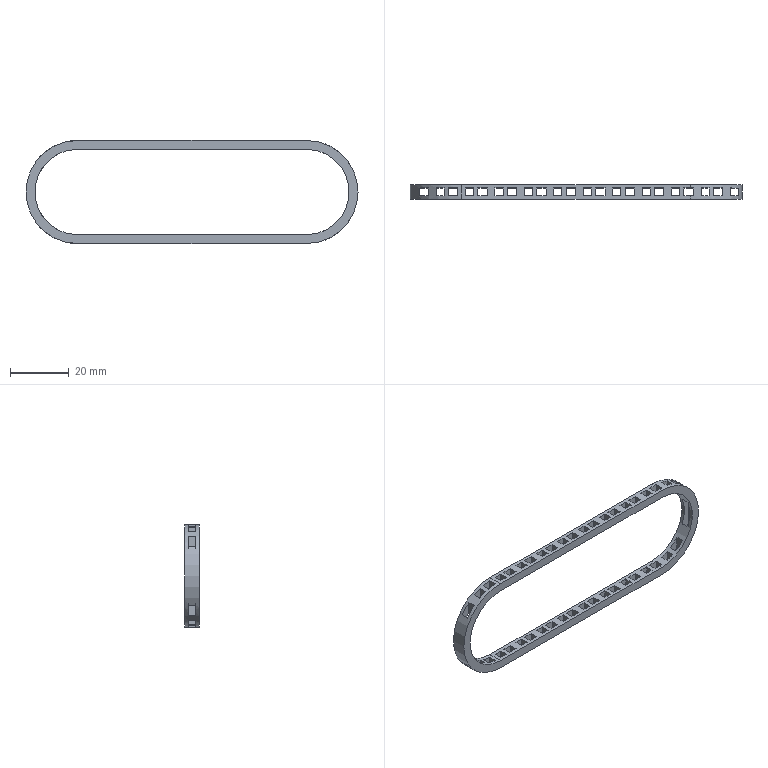Part | STEP file | 1/4in chain | 1 solid | 183 faces | box 112.8 x 5 x 35 mm | volume 2655 mm3 | plane 179 | cylinder 4 | commonest cylinder face diameters 29 x2 35 x2